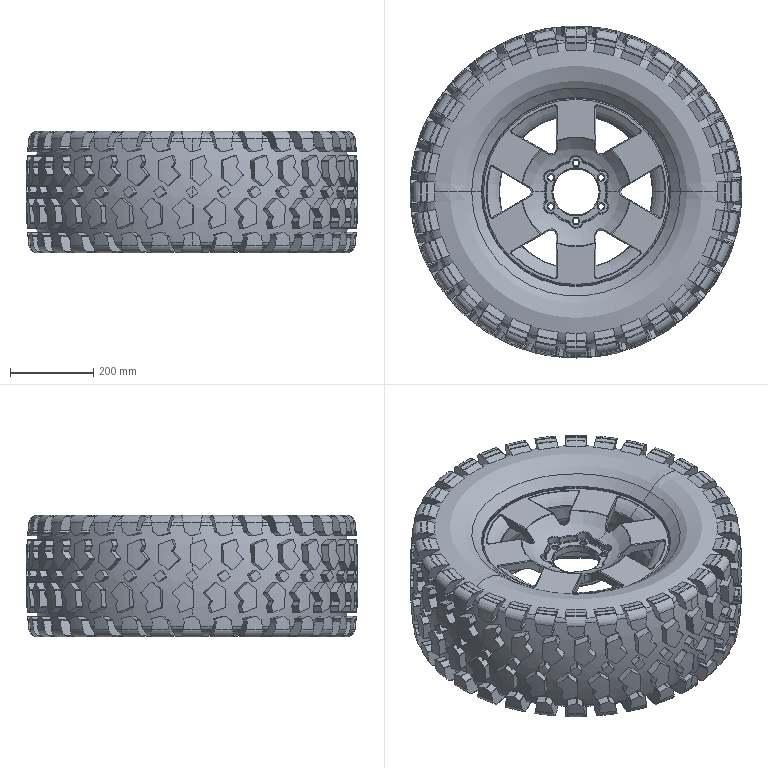Part | SolidWorks | features ICE 3, Revolution 3, Fillet 2, CirPattern 1, RevCut 1 | 1 solid | 3008 faces | volume 94107017 mm3 | cylinder 1296 | plane 985 | torus 496 | cone 151 | spline 48 | sphere 32 | commonest cylinder face diameters 4 x1234 9.821 x14 14 x12 34 x8 24 x7 150 x7